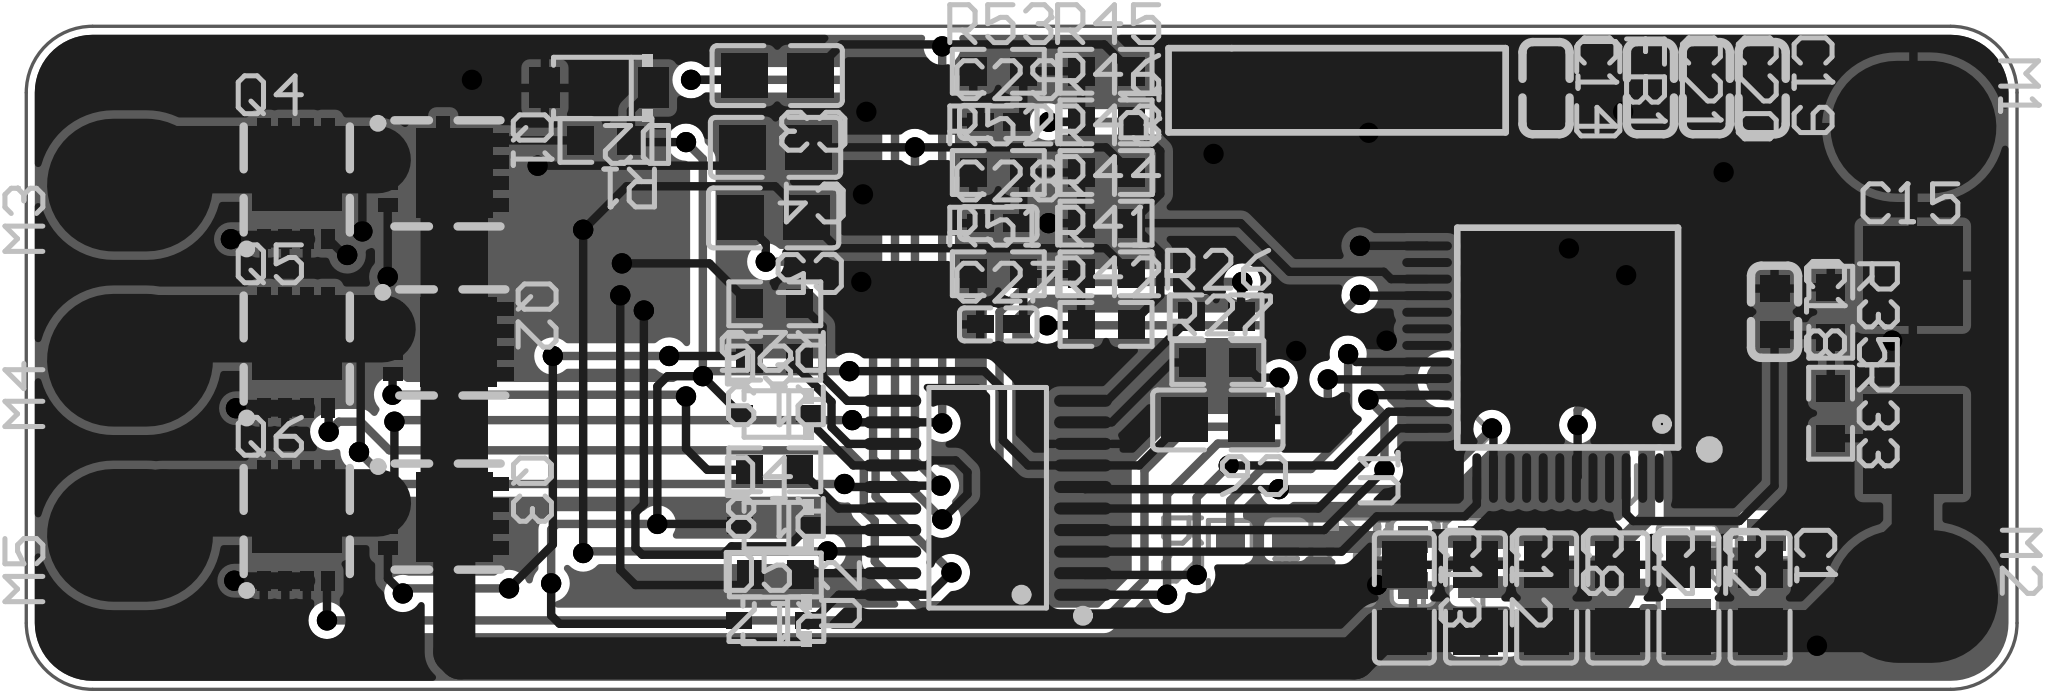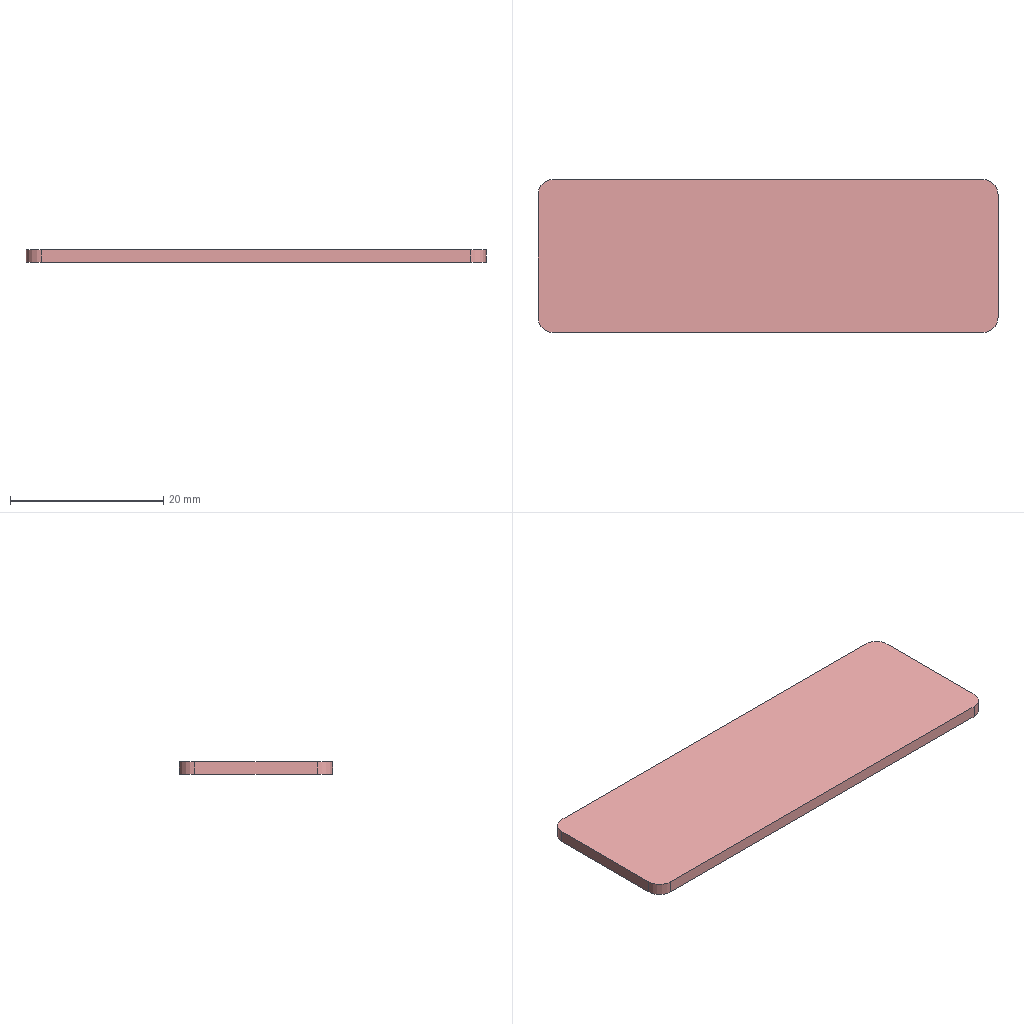Circuit board layout | Altium Designer | box 60 x 20 x 1.6 mm
Layer stack:
# Altium Designer layer stack of  (unit mm; dielectric type: 0 none, 1 core, 2 prepreg, 3 surface material)
index,name,kind,layer,copper_thickness_mm,dielectric_type,dielectric_thickness_mm,dielectric_material,dielectric_constant
0,Top Paste Mask Layer,other,,,,,,
1,Top Silkscreen Layer,other,,,,,,
2,Top Solder Mask Layer,dielectric,,,3,0.01,,3.3
3,Top Layer,copper,Top Layer,0.035,,,,
4,Dielectric1,dielectric,,,3,1.51,FR4,4.5
5,Bottom Layer,copper,Bottom Layer,0.035,,,,
6,Bottom Solder Mask Layer,dielectric,,,3,0.01,,3.3
7,Bottom Silkscreen Layer,other,,,,,,
8,Bottom Paste Mask Layer,other,,,,,,
# drill layer pairs: low layer,high layer
drill_pair,Top Layer,Bottom Layer
Part placement:
Designator,Comment,Layer,Footprint,Center-X(mm),Center-Y(mm),Rotation
C1,22uF,TopLayer,C0805,130.163,186.282,270
C2,22uF,TopLayer,C0805,128.018,186.282,270
C3,4.7uF,TopLayer,C0805,100.539,202.038,180
C4,4.7uF,TopLayer,C0805,100.489,199.874,180
C5,4.7uF,TopLayer,C0805,100.432,197.745,180
C6,22uF,TopLayer,C0805,113.819,191.65,180
C7,22uF,TopLayer,C0805,125.874,186.282,270
C8,22uF,TopLayer,C0805,123.729,186.282,270
C9,22uF,BottomLayer,C0805,127.997,186.55,90
C10,10uF,BottomLayer,C0603,119.701,187.359,90
C11,100nF,BottomLayer,C0603,117.91,187.353,90
C12,22uF,TopLayer,C0805,121.585,186.282,270
C13,22uF,TopLayer,C0805,119.44,186.282,270
C14,100nF,TopLayer,C0603,123.711,201.659,270
C15,470uf,TopLayer,焊盘,134.765,193.463,0
C18,100nF,TopLayer,C0603,130.598,194.914,270
C19,100nF,TopLayer,C0603,130.224,201.659,270
C20,10uF,TopLayer,C0603,128.541,201.659,270
C21,100nF,TopLayer,C0603,126.857,201.659,270
C27,100nF,TopLayer,C0402,107.202,194.533,0
C28,100nF,TopLayer,C0402,107.202,197.587,0
C29,100nF,TopLayer,C0402,107.202,200.642,0
D1,B5819WS,BottomLayer,SOD-323_L1.7-W1.3-LS2.5-FD,124.95,194.873,180
D2,BZT52C15,TopLayer,SOD-123_L2.7-W1.6-LS3.7-RD,95.174,201.665,180
D3,B5819WS,TopLayer,SOD-323_L1.7-W1.3-LS2.5-FD,100.467,191.831,0
D4,B5819WS,TopLayer,SOD-323_L1.7-W1.3-LS2.5-FD,100.467,188.463,0
D5,B5819WS,TopLayer,SOD-323_L1.7-W1.3-LS2.5-FD,100.432,185.604,0
D6,DSK34,BottomLayer,SOD-123_L2.8-W1.8-LS3.7-RD,130.343,186.499,270
FB1,MLB1608F-000T,TopLayer,L0603,125.285,201.643,270
M1,MountHole,TopLayer,3*4焊盘,134.784,200.482,270
M2,MountHole,TopLayer,3*4焊盘,134.835,186.324,270
M3,MountHole,TopLayer,3*4焊盘,81.033,198.736,90
M4,MountHole,TopLayer,3*4焊盘,81.033,193.452,90
M5,MountHole,TopLayer,3*4焊盘,81.033,188.169,90
P1,Header-D-M 1x4P,TopLayer,调试端口2.54_1X4,117.414,201.595,90
P2,Header-D-M 1x3P,BottomLayer,3P,121.34,194.862,0
Q1,TPN2R703NL,L1Q(M,TopLayer,TSON-8_L3.1-W3.1-P0.65-LS3.3-BL-EP,90.475,199.109,270
Q2,TPN2R703NL,L1Q(M,TopLayer,TSON-8_L3.1-W3.1-P0.65-LS3.3-BL-EP,90.621,194.009,270
Q3,TPN2R703NL,L1Q(M,TopLayer,TSON-8_L3.1-W3.1-P0.65-LS3.3-BL-EP,90.481,188.756,270
Q4,TPN2R703NL,L1Q(M,TopLayer,TSON-8_L3.1-W3.1-P0.65-LS3.3-BL-EP,86.039,198.779,0
Q5,TPN2R703NL,L1Q(M,TopLayer,TSON-8_L3.1-W3.1-P0.65-LS3.3-BL-EP,86.039,193.679,0
Q6,TPN2R703NL,L1Q(M,TopLayer,TSON-8_L3.1-W3.1-P0.65-LS3.3-BL-EP,86.039,188.477,0
R1,100Ω,TopLayer,R0603,95.378,200.083,180
R2,10kΩ,BottomLayer,R0603,114.194,187.235,270
R17,4.7Ω,TopLayer,R0603,100.482,186.976,180
R18,4.7Ω,TopLayer,R0603,100.467,190.147,180
R19,4.7Ω,TopLayer,R0603,100.467,193.514,180
R25,4.7Ω,TopLayer,R0603,100.467,195.155,180
R26,4.7Ω,TopLayer,R0603,113.768,194.761,0
R27,4.7Ω,TopLayer,R0603,113.819,193.384,0
R33,47kΩ,TopLayer,R0603,132.287,191.854,270
R34,100Ω,BottomLayer,R0603,124.848,192.883,180
R35,10kΩ,TopLayer,R0603,132.292,194.901,270
R41,5.1kΩ,TopLayer,R0603,110.451,196.06,0
R42,1kΩ,TopLayer,R0603,110.451,194.533,0
R43,5.1kΩ,TopLayer,R0603,110.451,199.114,0
R44,1kΩ,TopLayer,R0603,110.451,197.587,0
R45,5.1kΩ,TopLayer,R0603,110.451,202.169,0
R46,1kΩ,TopLayer,R0603,110.451,200.642,0
R51,1kΩ,TopLayer,R0603,107.202,196.06,0
R52,1kΩ,TopLayer,R0603,107.202,199.114,0
R53,1kΩ,TopLayer,R0603,107.202,202.169,0
STA,LTST-C191KSKT,BottomLayer,LED0603-RD-YELLOW,115.866,187.248,90
U1,STC32G8K64-42I-LQFP48,TopLayer,LQFP-48_L7.0-W7.0-P0.50-LS9.0-BL,124.376,194.149,90
U2,FD6288T,TopLayer,TSSOP-20_L6.5-W4.4-P0.65-LS6.4-BL,106.882,189.304,90
U3,SE8650KX-LF,BottomLayer,SOT-89-3_L4.3-W2.3-P1.50-LS4.3-BR,123.008,186.601,180
Pad and via stacks:
# Altium Designer via and pad stacks of  (unit mm). Each distinct definition once, with the count of objects using it.
# via: kind,start_layer,end_layer,hole_mm,diameter_mm,mode(0 simple;1 top-mid-bottom;2 full stack),diameter_per_layer,count,example_net
# pad: kind,layer,hole_mm,hole_type(0 round;1 square;2 slot),plating,top_size,top_shape(1 round;2 rect;3 octagon;9 rounded rect),mid_size,bottom_size,mode,footprint,size_per_layer,count,example
pad,Top Layer,0,0,plated,1.41x1.35,2,1.41x1.35,1.41x1.35,0,C0805,,20,C1.2
pad,Top Layer,0,0,plated,0.8x0.9,2,0.8x0.9,0.8x0.9,0,C0603,,10,C14.2
pad,Top Layer,0,0,plated,3x3,2,3x3,3x3,0,\u00BA\u00B8\u00C5\u00CC,,2,C15.1
pad,Top Layer,0,0,plated,0.7901x0.54,2,0.7901x0.54,0.7901x0.54,0,C0402,,6,C27.2
pad,Top Layer,0,0,plated,0.91x1.22,2,0.91x1.22,0.91x1.22,0,SOD-123_L2.7-W1.6-LS3.7-RD,,2,D2.2
pad,Top Layer,0,0,plated,0.78x0.5,2,0.78x0.5,0.78x0.5,0,SOD-323_L1.7-W1.3-LS2.5-FD,,6,D3.1
pad,Top Layer,0,0,plated,0.8x0.864,2,0.8x0.864,0.8x0.864,0,L0603,,2,FB1.1
pad,Top Layer,0,0,plated,4x5,1,4x5,4x5,0,3*4\u00BA\u00B8\u00C5\u00CC,,5,M1.1
pad,Top Layer,0,0,plated,1.575x1.575,1,1.575x1.575,1.575x1.575,0,\u00B5\u00F7\u00CA\u00D4\u00B6\u00CB\u00BF\u00DA2.54_1X4,,3,P1.4
pad,Top Layer,0,0,plated,1.575x1.575,2,1.575x1.575,1.575x1.575,0,\u00B5\u00F7\u00CA\u00D4\u00B6\u00CB\u00BF\u00DA2.54_1X4,,1,P1.1
pad,Top Layer,0,0,plated,0.6x0.4,2,0.6x0.4,0.6x0.4,0,TSON-8_L3.1-W3.1-P0.65-LS3.3-BL-EP,,24,Q1.1
pad,Top Layer,0,0,plated,0.4x0.6,2,0.4x0.6,0.4x0.6,0,TSON-8_L3.1-W3.1-P0.65-LS3.3-BL-EP,,36,Q1.8
pad,Top Layer,0,0,plated,2.7x2.3,2,2.7x2.3,2.7x2.3,0,TSON-8_L3.1-W3.1-P0.65-LS3.3-BL-EP,,6,Q1.9
pad,Top Layer,0,0,plated,0.8065x0.864,2,0.8065x0.864,0.8065x0.864,0,R0603,,36,R1.2
pad,Top Layer,0,0,plated,0.27x1.5,1,0.27x1.5,0.27x1.5,0,LQFP-48_L7.0-W7.0-P0.50-LS9.0-BL,,24,U1.1
pad,Top Layer,0,0,plated,1.5x0.27,1,1.5x0.27,1.5x0.27,0,LQFP-48_L7.0-W7.0-P0.50-LS9.0-BL,,24,U1.13
pad,Top Layer,0,0,plated,0.364x1.742,1,0.364x1.742,0.364x1.742,0,TSSOP-20_L6.5-W4.4-P0.65-LS6.4-BL,,20,U2.1
pad,Bottom Layer,0,0,plated,1.41x1.35,2,1.41x1.35,1.41x1.35,0,C0805,,2,C9.2
pad,Bottom Layer,0,0,plated,0.8x0.9,2,0.8x0.9,0.8x0.9,0,C0603,,4,C10.2
pad,Bottom Layer,0,0,plated,0.78x0.5,2,0.78x0.5,0.78x0.5,0,SOD-323_L1.7-W1.3-LS2.5-FD,,2,D1.1
pad,Bottom Layer,0,0,plated,0.95x1.15,2,0.95x1.15,0.95x1.15,0,SOD-123_L2.8-W1.8-LS3.7-RD,,2,D6.2
pad,Bottom Layer,0,0,plated,2.5x1.25,1,2.5x1.25,2.5x1.25,0,3P,,3,P2.1
pad,Bottom Layer,0,0,plated,0.8065x0.864,2,0.8065x0.864,0.8065x0.864,0,R0603,,4,R2.2
pad,Bottom Layer,0,0,plated,0.8x0.8,2,0.8x0.8,0.8x0.8,0,LED0603-RD-YELLOW,,2,STA.1
pad,Bottom Layer,0,0,plated,0.95x0.95,1,0.95x0.95,0.95x0.95,0,SOT-89-3_L4.3-W2.3-P1.50-LS4.3-BR,,1,U3.2
pad,Bottom Layer,0,0,plated,1.575x0.672,2,1.575x0.672,1.575x0.672,0,SOT-89-3_L4.3-W2.3-P1.50-LS4.3-BR,,2,U3.3
via,Top Layer,Bottom Layer,0.3048,0.61,0,,70,CBMF
Copper pours:
name,layer,net,type(0 solid;1 hatched;2 none)
Top Layer-GND,Top Layer,GND,0
Bottom Layer-GND,Bottom Layer,GND,0
Design rules, without the lines most boards share:
# Altium Designer design rules of  (exported by Altium Designer, unit mm)
# columns: name | kind | enabled | priority | scope1 | scope2 | descriptor | typed fields (field=value)
solderMaskExpansion | 13 | enabled | 2 | All | All | Solder Mask Expansion (Expansion =2.008mil) (All) | expansion=0.051